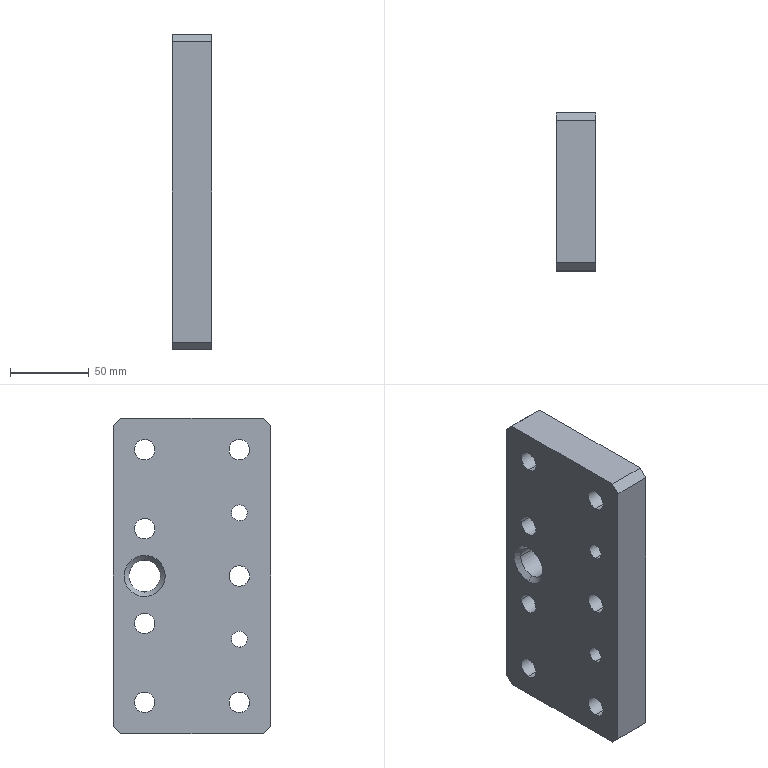Part | STEP file | Positioning_id1098_x_t | 1 solid | 55 faces | box 25 x 100 x 200 mm | volume 444348 mm3 | cylinder 34 | plane 17 | cone 4 | commonest cylinder face diameters 20 x16 13 x14 10 x4